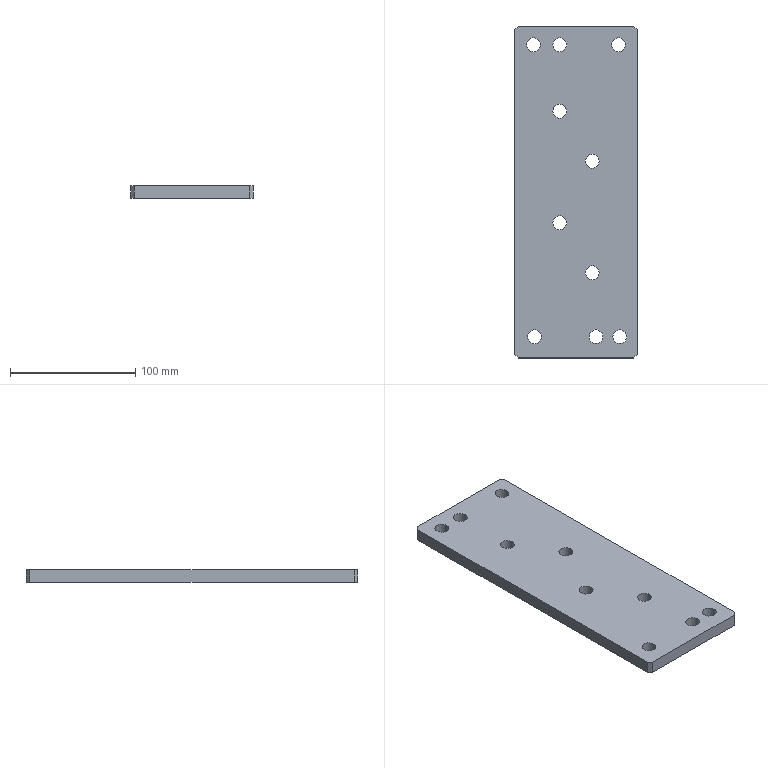Part | STEP file | 1_id190_x_t | 1 solid | 20 faces | box 98 x 265 x 10 mm | volume 250017 mm3 | cylinder 10 | plane 10 | commonest cylinder face diameters 11 x10